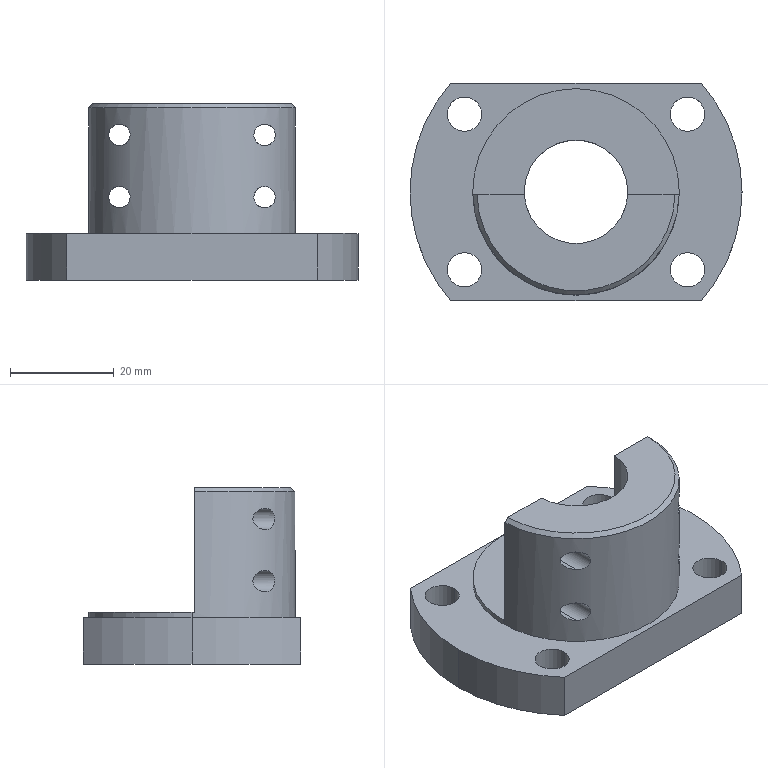Part | STEP file | _GAY12-D20-001.stp | 1 solid | 32 faces | box 64 x 42 x 34 mm | volume 29366 mm3 | cylinder 23 | plane 8 | cone 1 | commonest cylinder face diameters 4.134 x8 6.6 x8 64 x3 20 x2 39.8 x2